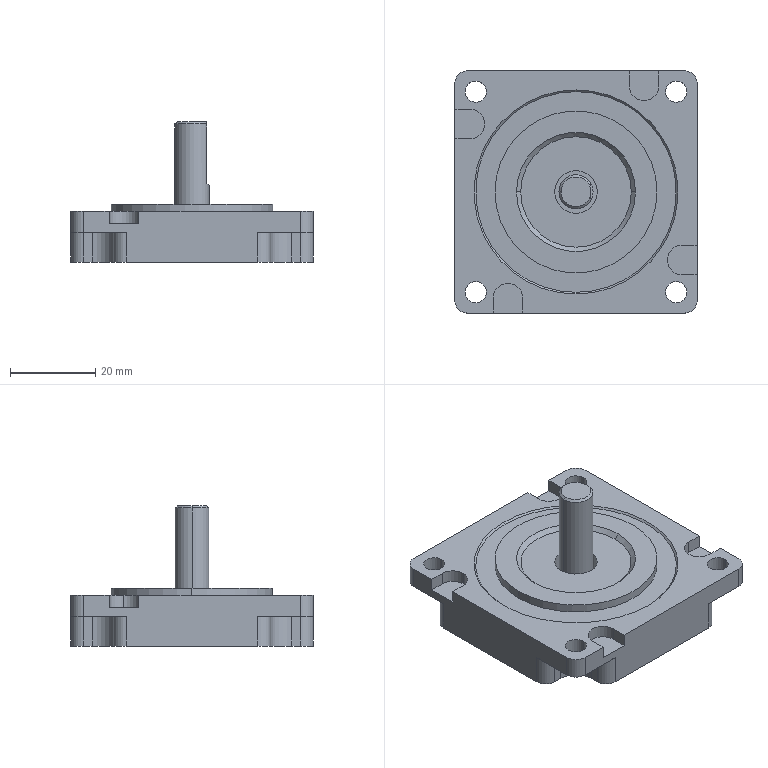Part | SolidWorks | features BaseBody 1 | 1 solid | 78 faces | box 57 x 57 x 33 mm | volume 37132 mm3 | plane 37 | cylinder 35 | cone 6 | commonest cylinder face diameters 6 x12 5 x8 10 x6 7 x5 8 x2 38.1 x2